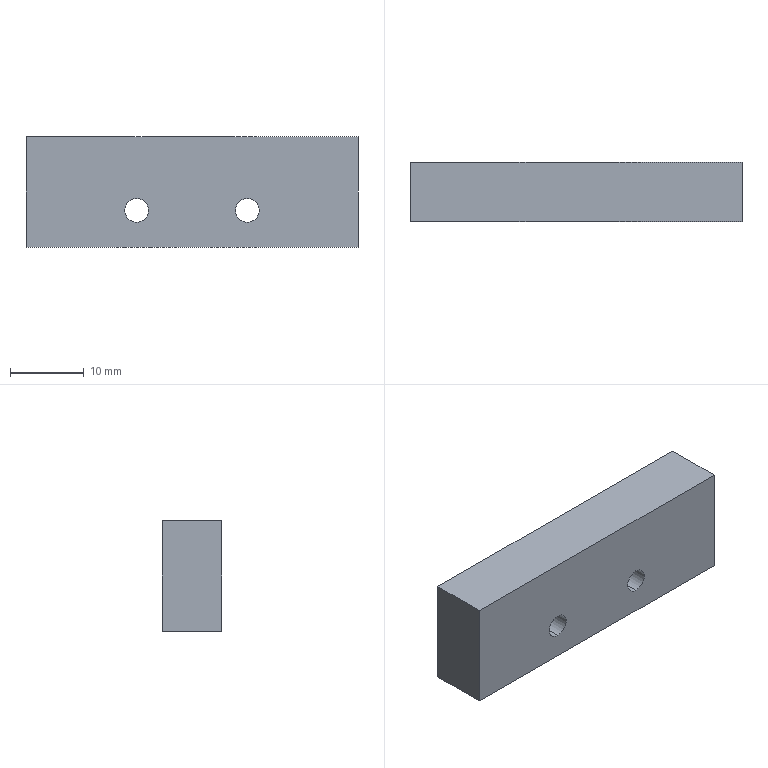Part | SolidWorks | features Extrusion 1, HoleWzd 1, ICE 1 | 1 solid | 16 faces | box 45 x 8 x 15 mm | volume 5130 mm3 | cylinder 8 | plane 8 | commonest cylinder face diameters 3.2 x4 6 x4
STEP:
#1=CARTESIAN_POINT('',(-7.5,4.5,-3.));
#2=VERTEX_POINT('',#1);
#3=CARTESIAN_POINT('',(-7.5,4.5,3.));
#4=VERTEX_POINT('',#3);
#5=CARTESIAN_POINT('',(-7.5,4.5,0.));
#6=DIRECTION('',(0.,1.,0.));
#7=DIRECTION('',(0.,0.,1.));
#8=AXIS2_PLACEMENT_3D('',#5,#6,#7);
#9=CIRCLE('',#8,3.);
#10=EDGE_CURVE('',#2,#4,#9,.T.);
#11=ORIENTED_EDGE('',*,*,#10,.F.);
#12=CARTESIAN_POINT('',(-7.5,8.,-3.));
#13=VERTEX_POINT('',#12);
#14=CARTESIAN_POINT('',(-7.5,8.,-3.));
#15=DIRECTION('',(0.,1.,0.));
#16=VECTOR('',#15,1000.);
#17=LINE('',#14,#16);
#18=EDGE_CURVE('',#2,#13,#17,.T.);
#19=ORIENTED_EDGE('',*,*,#18,.T.);
#20=CARTESIAN_POINT('',(-7.5,8.,3.));
#21=VERTEX_POINT('',#20);
#22=CARTESIAN_POINT('',(-7.5,8.,0.));
#23=DIRECTION('',(0.,1.,0.));
#24=DIRECTION('',(0.,0.,1.));
#25=AXIS2_PLACEMENT_3D('',#22,#23,#24);
#26=CIRCLE('',#25,3.);
#27=EDGE_CURVE('',#13,#21,#26,.T.);
#28=ORIENTED_EDGE('',*,*,#27,.T.);
#29=CARTESIAN_POINT('',(-7.5,8.,3.));
#30=DIRECTION('',(0.,1.,0.));
#31=VECTOR('',#30,1000.);
#32=LINE('',#29,#31);
#33=EDGE_CURVE('',#4,#21,#32,.T.);
#34=ORIENTED_EDGE('',*,*,#33,.F.);
#35=EDGE_LOOP('',(#11,#19,#28,#34));
#36=FACE_OUTER_BOUND('',#35,.T.);
#37=CARTESIAN_POINT('',(-7.5,8.,0.));
#38=DIRECTION('',(0.,1.,0.));
#39=DIRECTION('',(0.,0.,1.));
#40=AXIS2_PLACEMENT_3D('',#37,#38,#39);
#41=CYLINDRICAL_SURFACE('',#40,3.);
#42=ADVANCED_FACE('',(#36),#41,.F.);
#43=CARTESIAN_POINT('',(-7.5,0.,-1.6));
#44=VERTEX_POINT('',#43);
#45=CARTESIAN_POINT('',(-7.5,0.,1.6));
#46=VERTEX_POINT('',#45);
#47=CARTESIAN_POINT('',(-7.5,0.,0.));
#48=DIRECTION('',(0.,1.,0.));
#49=DIRECTION('',(0.,0.,1.));
#50=AXIS2_PLACEMENT_3D('',#47,#48,#49);
#51=CIRCLE('',#50,1.6);
#52=EDGE_CURVE('',#44,#46,#51,.T.);
#53=ORIENTED_EDGE('',*,*,#52,.F.);
#54=CARTESIAN_POINT('',(-7.5,4.5,-1.6));
#55=VERTEX_POINT('',#54);
#56=CARTESIAN_POINT('',(-7.5,8.,-1.6));
#57=DIRECTION('',(0.,1.,0.));
#58=VECTOR('',#57,1000.);
#59=LINE('',#56,#58);
#60=EDGE_CURVE('',#44,#55,#59,.T.);
#61=ORIENTED_EDGE('',*,*,#60,.T.);
#62=CARTESIAN_POINT('',(-7.5,4.5,1.6));
#63=VERTEX_POINT('',#62);
#64=CARTESIAN_POINT('',(-7.5,4.5,0.));
#65=DIRECTION('',(0.,1.,0.));
#66=DIRECTION('',(0.,0.,1.));
#67=AXIS2_PLACEMENT_3D('',#64,#65,#66);
#68=CIRCLE('',#67,1.6);
#69=EDGE_CURVE('',#55,#63,#68,.T.);
#70=ORIENTED_EDGE('',*,*,#69,.T.);
#71=CARTESIAN_POINT('',(-7.5,8.,1.6));
#72=DIRECTION('',(0.,1.,0.));
#73=VECTOR('',#72,1000.);
#74=LINE('',#71,#73);
#75=EDGE_CURVE('',#46,#63,#74,.T.);
#76=ORIENTED_EDGE('',*,*,#75,.F.);
#77=EDGE_LOOP('',(#53,#61,#70,#76));
#78=FACE_OUTER_BOUND('',#77,.T.);
#79=CARTESIAN_POINT('',(-7.5,8.,0.));
#80=DIRECTION('',(0.,1.,0.));
#81=DIRECTION('',(0.,0.,1.));
#82=AXIS2_PLACEMENT_3D('',#79,#80,#81);
#83=CYLINDRICAL_SURFACE('',#82,1.6);
#84=ADVANCED_FACE('',(#78),#83,.F.);
#85=CARTESIAN_POINT('',(7.5,4.5,-3.));
#86=VERTEX_POINT('',#85);
#87=CARTESIAN_POINT('',(7.5,4.5,3.));
#88=VERTEX_POINT('',#87);
#89=CARTESIAN_POINT('',(7.5,4.5,0.));
#90=DIRECTION('',(0.,1.,0.));
#91=DIRECTION('',(0.,0.,1.));
#92=AXIS2_PLACEMENT_3D('',#89,#90,#91);
#93=CIRCLE('',#92,3.);
#94=EDGE_CURVE('',#86,#88,#93,.T.);
#95=ORIENTED_EDGE('',*,*,#94,.F.);
#96=CARTESIAN_POINT('',(7.5,8.,-3.));
#97=VERTEX_POINT('',#96);
#98=CARTESIAN_POINT('',(7.5,8.,-3.));
#99=DIRECTION('',(0.,1.,0.));
#100=VECTOR('',#99,1000.);
#101=LINE('',#98,#100);
#102=EDGE_CURVE('',#86,#97,#101,.T.);
#103=ORIENTED_EDGE('',*,*,#102,.T.);
#104=CARTESIAN_POINT('',(7.5,8.,3.));
#105=VERTEX_POINT('',#104);
#106=CARTESIAN_POINT('',(7.5,8.,0.));
#107=DIRECTION('',(0.,1.,0.));
#108=DIRECTION('',(0.,0.,1.));
#109=AXIS2_PLACEMENT_3D('',#106,#107,#108);
#110=CIRCLE('',#109,3.);
#111=EDGE_CURVE('',#97,#105,#110,.T.);
#112=ORIENTED_EDGE('',*,*,#111,.T.);
#113=CARTESIAN_POINT('',(7.5,8.,3.));
#114=DIRECTION('',(0.,1.,0.));
#115=VECTOR('',#114,1000.);
#116=LINE('',#113,#115);
#117=EDGE_CURVE('',#88,#105,#116,.T.);
#118=ORIENTED_EDGE('',*,*,#117,.F.);
#119=EDGE_LOOP('',(#95,#103,#112,#118));
#120=FACE_OUTER_BOUND('',#119,.T.);
#121=CARTESIAN_POINT('',(7.5,8.,0.));
#122=DIRECTION('',(0.,1.,0.));
#123=DIRECTION('',(0.,0.,1.));
#124=AXIS2_PLACEMENT_3D('',#121,#122,#123);
#125=CYLINDRICAL_SURFACE('',#124,3.);
#126=ADVANCED_FACE('',(#120),#125,.F.);
#127=CARTESIAN_POINT('',(7.5,0.,-1.6));
#128=VERTEX_POINT('',#127);
#129=CARTESIAN_POINT('',(7.5,0.,1.6));
#130=VERTEX_POINT('',#129);
#131=CARTESIAN_POINT('',(7.5,0.,0.));
#132=DIRECTION('',(0.,1.,0.));
#133=DIRECTION('',(0.,0.,1.));
#134=AXIS2_PLACEMENT_3D('',#131,#132,#133);
#135=CIRCLE('',#134,1.6);
#136=EDGE_CURVE('',#128,#130,#135,.T.);
#137=ORIENTED_EDGE('',*,*,#136,.F.);
#138=CARTESIAN_POINT('',(7.5,4.5,-1.6));
#139=VERTEX_POINT('',#138);
#140=CARTESIAN_POINT('',(7.5,8.,-1.6));
#141=DIRECTION('',(0.,1.,0.));
#142=VECTOR('',#141,1000.);
#143=LINE('',#140,#142);
#144=EDGE_CURVE('',#128,#139,#143,.T.);
#145=ORIENTED_EDGE('',*,*,#144,.T.);
#146=CARTESIAN_POINT('',(7.5,4.5,1.6));
#147=VERTEX_POINT('',#146);
#148=CARTESIAN_POINT('',(7.5,4.5,0.));
#149=DIRECTION('',(0.,1.,0.));
#150=DIRECTION('',(0.,0.,1.));
#151=AXIS2_PLACEMENT_3D('',#148,#149,#150);
#152=CIRCLE('',#151,1.6);
#153=EDGE_CURVE('',#139,#147,#152,.T.);
#154=ORIENTED_EDGE('',*,*,#153,.T.);
#155=CARTESIAN_POINT('',(7.5,8.,1.6));
#156=DIRECTION('',(0.,1.,0.));
#157=VECTOR('',#156,1000.);
#158=LINE('',#155,#157);
#159=EDGE_CURVE('',#130,#147,#158,.T.);
#160=ORIENTED_EDGE('',*,*,#159,.F.);
#161=EDGE_LOOP('',(#137,#145,#154,#160));
#162=FACE_OUTER_BOUND('',#161,.T.);
#163=CARTESIAN_POINT('',(7.5,8.,0.));
#164=DIRECTION('',(0.,1.,0.));
#165=DIRECTION('',(0.,0.,1.));
#166=AXIS2_PLACEMENT_3D('',#163,#164,#165);
#167=CYLINDRICAL_SURFACE('',#166,1.6);
#168=ADVANCED_FACE('',(#162),#167,.F.);
#169=CARTESIAN_POINT('',(22.5,0.,10.));
#170=VERTEX_POINT('',#169);
#171=CARTESIAN_POINT('',(22.5,0.,-5.));
#172=VERTEX_POINT('',#171);
#173=CARTESIAN_POINT('',(22.5,0.,-5.));
#174=DIRECTION('',(0.,0.,-1.));
#175=VECTOR('',#174,1000.);
#176=LINE('',#173,#175);
#177=EDGE_CURVE('',#170,#172,#176,.T.);
#178=ORIENTED_EDGE('',*,*,#177,.T.);
#179=CARTESIAN_POINT('',(22.5,8.,-5.));
#180=VERTEX_POINT('',#179);
#181=CARTESIAN_POINT('',(22.5,8.,-5.));
#182=DIRECTION('',(0.,-1.,0.));
#183=VECTOR('',#182,1000.);
#184=LINE('',#181,#183);
#185=EDGE_CURVE('',#180,#172,#184,.T.);
#186=ORIENTED_EDGE('',*,*,#185,.F.);
#187=CARTESIAN_POINT('',(22.5,8.,10.));
#188=VERTEX_POINT('',#187);
#189=CARTESIAN_POINT('',(22.5,8.,-5.));
#190=DIRECTION('',(0.,0.,-1.));
#191=VECTOR('',#190,1000.);
#192=LINE('',#189,#191);
#193=EDGE_CURVE('',#188,#180,#192,.T.);
#194=ORIENTED_EDGE('',*,*,#193,.F.);
#195=CARTESIAN_POINT('',(22.5,0.,10.));
#196=DIRECTION('',(0.,1.,0.));
#197=VECTOR('',#196,1000.);
#198=LINE('',#195,#197);
#199=EDGE_CURVE('',#170,#188,#198,.T.);
#200=ORIENTED_EDGE('',*,*,#199,.F.);
#201=EDGE_LOOP('',(#178,#186,#194,#200));
#202=FACE_OUTER_BOUND('',#201,.T.);
#203=CARTESIAN_POINT('',(22.5,8.,-5.));
#204=DIRECTION('',(-1.,0.,0.));
#205=DIRECTION('',(0.,0.,1.));
#206=AXIS2_PLACEMENT_3D('',#203,#204,#205);
#207=PLANE('',#206);
#208=ADVANCED_FACE('',(#202),#207,.F.);
#209=CARTESIAN_POINT('',(-22.5,0.,-5.));
#210=VERTEX_POINT('',#209);
#211=CARTESIAN_POINT('',(-22.5,0.,-5.));
#212=DIRECTION('',(-1.,0.,0.));
#213=VECTOR('',#212,1000.);
#214=LINE('',#211,#213);
#215=EDGE_CURVE('',#172,#210,#214,.T.);
#216=ORIENTED_EDGE('',*,*,#215,.T.);
#217=CARTESIAN_POINT('',(-22.5,8.,-5.));
#218=VERTEX_POINT('',#217);
#219=CARTESIAN_POINT('',(-22.5,8.,-5.));
#220=DIRECTION('',(0.,-1.,0.));
#221=VECTOR('',#220,1000.);
#222=LINE('',#219,#221);
#223=EDGE_CURVE('',#218,#210,#222,.T.);
#224=ORIENTED_EDGE('',*,*,#223,.F.);
#225=CARTESIAN_POINT('',(-22.5,8.,-5.));
#226=DIRECTION('',(-1.,0.,0.));
#227=VECTOR('',#226,1000.);
#228=LINE('',#225,#227);
#229=EDGE_CURVE('',#180,#218,#228,.T.);
#230=ORIENTED_EDGE('',*,*,#229,.F.);
#231=ORIENTED_EDGE('',*,*,#185,.T.);
#232=EDGE_LOOP('',(#216,#224,#230,#231));
#233=FACE_OUTER_BOUND('',#232,.T.);
#234=CARTESIAN_POINT('',(-22.5,8.,-5.));
#235=DIRECTION('',(0.,0.,1.));
#236=DIRECTION('',(1.,0.,0.));
#237=AXIS2_PLACEMENT_3D('',#234,#235,#236);
#238=PLANE('',#237);
#239=ADVANCED_FACE('',(#233),#238,.F.);
#240=CARTESIAN_POINT('',(-22.5,0.,10.));
#241=VERTEX_POINT('',#240);
#242=CARTESIAN_POINT('',(-22.5,0.,-5.));
#243=DIRECTION('',(0.,0.,1.));
#244=VECTOR('',#243,1000.);
#245=LINE('',#242,#244);
#246=EDGE_CURVE('',#210,#241,#245,.T.);
#247=ORIENTED_EDGE('',*,*,#246,.T.);
#248=CARTESIAN_POINT('',(-22.5,8.,10.));
#249=VERTEX_POINT('',#248);
#250=CARTESIAN_POINT('',(-22.5,8.,10.));
#251=DIRECTION('',(0.,-1.,0.));
#252=VECTOR('',#251,1000.);
#253=LINE('',#250,#252);
#254=EDGE_CURVE('',#249,#241,#253,.T.);
#255=ORIENTED_EDGE('',*,*,#254,.F.);
#256=CARTESIAN_POINT('',(-22.5,8.,-5.));
#257=DIRECTION('',(0.,0.,1.));
#258=VECTOR('',#257,1000.);
#259=LINE('',#256,#258);
#260=EDGE_CURVE('',#218,#249,#259,.T.);
#261=ORIENTED_EDGE('',*,*,#260,.F.);
#262=ORIENTED_EDGE('',*,*,#223,.T.);
#263=EDGE_LOOP('',(#247,#255,#261,#262));
#264=FACE_OUTER_BOUND('',#263,.T.);
#265=CARTESIAN_POINT('',(-22.5,8.,-5.));
#266=DIRECTION('',(1.,0.,0.));
#267=DIRECTION('',(0.,0.,-1.));
#268=AXIS2_PLACEMENT_3D('',#265,#266,#267);
#269=PLANE('',#268);
#270=ADVANCED_FACE('',(#264),#269,.F.);
#271=CARTESIAN_POINT('',(-7.5,8.,0.));
#272=DIRECTION('',(0.,1.,0.));
#273=DIRECTION('',(0.,0.,1.));
#274=AXIS2_PLACEMENT_3D('',#271,#272,#273);
#275=CIRCLE('',#274,3.);
#276=EDGE_CURVE('',#21,#13,#275,.T.);
#277=ORIENTED_EDGE('',*,*,#276,.F.);
#278=ORIENTED_EDGE('',*,*,#27,.F.);
#279=EDGE_LOOP('',(#277,#278));
#280=FACE_BOUND('',#279,.T.);
#281=CARTESIAN_POINT('',(7.5,8.,0.));
#282=DIRECTION('',(0.,1.,0.));
#283=DIRECTION('',(0.,0.,1.));
#284=AXIS2_PLACEMENT_3D('',#281,#282,#283);
#285=CIRCLE('',#284,3.);
#286=EDGE_CURVE('',#105,#97,#285,.T.);
#287=ORIENTED_EDGE('',*,*,#286,.F.);
#288=ORIENTED_EDGE('',*,*,#111,.F.);
#289=EDGE_LOOP('',(#287,#288));
#290=FACE_BOUND('',#289,.T.);
#291=ORIENTED_EDGE('',*,*,#193,.T.);
#292=ORIENTED_EDGE('',*,*,#229,.T.);
#293=ORIENTED_EDGE('',*,*,#260,.T.);
#294=CARTESIAN_POINT('',(22.5,8.,10.));
#295=DIRECTION('',(-1.,0.,0.));
#296=VECTOR('',#295,1000.);
#297=LINE('',#294,#296);
#298=EDGE_CURVE('',#188,#249,#297,.T.);
#299=ORIENTED_EDGE('',*,*,#298,.F.);
#300=EDGE_LOOP('',(#291,#292,#293,#299));
#301=FACE_OUTER_BOUND('',#300,.T.);
#302=CARTESIAN_POINT('',(0.,8.,0.));
#303=DIRECTION('',(0.,1.,0.));
#304=DIRECTION('',(0.,0.,1.));
#305=AXIS2_PLACEMENT_3D('',#302,#303,#304);
#306=PLANE('',#305);
#307=ADVANCED_FACE('',(#280,#290,#301),#306,.T.);
#308=CARTESIAN_POINT('',(-7.5,0.,0.));
#309=DIRECTION('',(0.,1.,0.));
#310=DIRECTION('',(0.,0.,1.));
#311=AXIS2_PLACEMENT_3D('',#308,#309,#310);
#312=CIRCLE('',#311,1.6);
#313=EDGE_CURVE('',#46,#44,#312,.T.);
#314=ORIENTED_EDGE('',*,*,#313,.T.);
#315=ORIENTED_EDGE('',*,*,#52,.T.);
#316=EDGE_LOOP('',(#314,#315));
#317=FACE_BOUND('',#316,.T.);
#318=CARTESIAN_POINT('',(7.5,0.,0.));
#319=DIRECTION('',(0.,1.,0.));
#320=DIRECTION('',(0.,0.,1.));
#321=AXIS2_PLACEMENT_3D('',#318,#319,#320);
#322=CIRCLE('',#321,1.6);
#323=EDGE_CURVE('',#130,#128,#322,.T.);
#324=ORIENTED_EDGE('',*,*,#323,.T.);
#325=ORIENTED_EDGE('',*,*,#136,.T.);
#326=EDGE_LOOP('',(#324,#325));
#327=FACE_BOUND('',#326,.T.);
#328=ORIENTED_EDGE('',*,*,#177,.F.);
#329=CARTESIAN_POINT('',(-22.5,0.,10.));
#330=DIRECTION('',(1.,0.,0.));
#331=VECTOR('',#330,1000.);
#332=LINE('',#329,#331);
#333=EDGE_CURVE('',#241,#170,#332,.T.);
#334=ORIENTED_EDGE('',*,*,#333,.F.);
#335=ORIENTED_EDGE('',*,*,#246,.F.);
#336=ORIENTED_EDGE('',*,*,#215,.F.);
#337=EDGE_LOOP('',(#328,#334,#335,#336));
#338=FACE_OUTER_BOUND('',#337,.T.);
#339=CARTESIAN_POINT('',(0.,0.,0.));
#340=DIRECTION('',(0.,1.,0.));
#341=DIRECTION('',(0.,0.,1.));
#342=AXIS2_PLACEMENT_3D('',#339,#340,#341);
#343=PLANE('',#342);
#344=ADVANCED_FACE('',(#317,#327,#338),#343,.F.);
#345=ORIENTED_EDGE('',*,*,#144,.F.);
#346=ORIENTED_EDGE('',*,*,#323,.F.);
#347=ORIENTED_EDGE('',*,*,#159,.T.);
#348=CARTESIAN_POINT('',(7.5,4.5,0.));
#349=DIRECTION('',(0.,1.,0.));
#350=DIRECTION('',(0.,0.,1.));
#351=AXIS2_PLACEMENT_3D('',#348,#349,#350);
#352=CIRCLE('',#351,1.6);
#353=EDGE_CURVE('',#147,#139,#352,.T.);
#354=ORIENTED_EDGE('',*,*,#353,.T.);
#355=EDGE_LOOP('',(#345,#346,#347,#354));
#356=FACE_OUTER_BOUND('',#355,.T.);
#357=CARTESIAN_POINT('',(7.5,8.,0.));
#358=DIRECTION('',(0.,1.,0.));
#359=DIRECTION('',(0.,0.,1.));
#360=AXIS2_PLACEMENT_3D('',#357,#358,#359);
#361=CYLINDRICAL_SURFACE('',#360,1.6);
#362=ADVANCED_FACE('',(#356),#361,.F.);
#363=ORIENTED_EDGE('',*,*,#353,.F.);
#364=ORIENTED_EDGE('',*,*,#153,.F.);
#365=EDGE_LOOP('',(#363,#364));
#366=FACE_BOUND('',#365,.T.);
#367=CARTESIAN_POINT('',(7.5,4.5,0.));
#368=DIRECTION('',(0.,1.,0.));
#369=DIRECTION('',(0.,0.,1.));
#370=AXIS2_PLACEMENT_3D('',#367,#368,#369);
#371=CIRCLE('',#370,3.);
#372=EDGE_CURVE('',#88,#86,#371,.T.);
#373=ORIENTED_EDGE('',*,*,#372,.T.);
#374=ORIENTED_EDGE('',*,*,#94,.T.);
#375=EDGE_LOOP('',(#373,#374));
#376=FACE_OUTER_BOUND('',#375,.T.);
#377=CARTESIAN_POINT('',(9.1,4.5,0.));
#378=DIRECTION('',(0.,-1.,0.));
#379=DIRECTION('',(0.,0.,-1.));
#380=AXIS2_PLACEMENT_3D('',#377,#378,#379);
#381=PLANE('',#380);
#382=ADVANCED_FACE('',(#366,#376),#381,.F.);
#383=ORIENTED_EDGE('',*,*,#102,.F.);
#384=ORIENTED_EDGE('',*,*,#372,.F.);
#385=ORIENTED_EDGE('',*,*,#117,.T.);
#386=ORIENTED_EDGE('',*,*,#286,.T.);
#387=EDGE_LOOP('',(#383,#384,#385,#386));
#388=FACE_OUTER_BOUND('',#387,.T.);
#389=CARTESIAN_POINT('',(7.5,8.,0.));
#390=DIRECTION('',(0.,1.,0.));
#391=DIRECTION('',(0.,0.,1.));
#392=AXIS2_PLACEMENT_3D('',#389,#390,#391);
#393=CYLINDRICAL_SURFACE('',#392,3.);
#394=ADVANCED_FACE('',(#388),#393,.F.);
#395=ORIENTED_EDGE('',*,*,#60,.F.);
#396=ORIENTED_EDGE('',*,*,#313,.F.);
#397=ORIENTED_EDGE('',*,*,#75,.T.);
#398=CARTESIAN_POINT('',(-7.5,4.5,0.));
#399=DIRECTION('',(0.,1.,0.));
#400=DIRECTION('',(0.,0.,1.));
#401=AXIS2_PLACEMENT_3D('',#398,#399,#400);
#402=CIRCLE('',#401,1.6);
#403=EDGE_CURVE('',#63,#55,#402,.T.);
#404=ORIENTED_EDGE('',*,*,#403,.T.);
#405=EDGE_LOOP('',(#395,#396,#397,#404));
#406=FACE_OUTER_BOUND('',#405,.T.);
#407=CARTESIAN_POINT('',(-7.5,8.,0.));
#408=DIRECTION('',(0.,1.,0.));
#409=DIRECTION('',(0.,0.,1.));
#410=AXIS2_PLACEMENT_3D('',#407,#408,#409);
#411=CYLINDRICAL_SURFACE('',#410,1.6);
#412=ADVANCED_FACE('',(#406),#411,.F.);
#413=ORIENTED_EDGE('',*,*,#403,.F.);
#414=ORIENTED_EDGE('',*,*,#69,.F.);
#415=EDGE_LOOP('',(#413,#414));
#416=FACE_BOUND('',#415,.T.);
#417=CARTESIAN_POINT('',(-7.5,4.5,0.));
#418=DIRECTION('',(0.,1.,0.));
#419=DIRECTION('',(0.,0.,1.));
#420=AXIS2_PLACEMENT_3D('',#417,#418,#419);
#421=CIRCLE('',#420,3.);
#422=EDGE_CURVE('',#4,#2,#421,.T.);
#423=ORIENTED_EDGE('',*,*,#422,.T.);
#424=ORIENTED_EDGE('',*,*,#10,.T.);
#425=EDGE_LOOP('',(#423,#424));
#426=FACE_OUTER_BOUND('',#425,.T.);
#427=CARTESIAN_POINT('',(-5.9,4.5,0.));
#428=DIRECTION('',(0.,-1.,0.));
#429=DIRECTION('',(0.,0.,-1.));
#430=AXIS2_PLACEMENT_3D('',#427,#428,#429);
#431=PLANE('',#430);
#432=ADVANCED_FACE('',(#416,#426),#431,.F.);
#433=ORIENTED_EDGE('',*,*,#18,.F.);
#434=ORIENTED_EDGE('',*,*,#422,.F.);
#435=ORIENTED_EDGE('',*,*,#33,.T.);
#436=ORIENTED_EDGE('',*,*,#276,.T.);
#437=EDGE_LOOP('',(#433,#434,#435,#436));
#438=FACE_OUTER_BOUND('',#437,.T.);
#439=CARTESIAN_POINT('',(-7.5,8.,0.));
#440=DIRECTION('',(0.,1.,0.));
#441=DIRECTION('',(0.,0.,1.));
#442=AXIS2_PLACEMENT_3D('',#439,#440,#441);
#443=CYLINDRICAL_SURFACE('',#442,3.);
#444=ADVANCED_FACE('',(#438),#443,.F.);
#445=ORIENTED_EDGE('',*,*,#254,.T.);
#446=ORIENTED_EDGE('',*,*,#333,.T.);
#447=ORIENTED_EDGE('',*,*,#199,.T.);
#448=ORIENTED_EDGE('',*,*,#298,.T.);
#449=EDGE_LOOP('',(#445,#446,#447,#448));
#450=FACE_OUTER_BOUND('',#449,.T.);
#451=CARTESIAN_POINT('',(0.,0.,10.));
#452=DIRECTION('',(0.,0.,1.));
#453=DIRECTION('',(1.,0.,0.));
#454=AXIS2_PLACEMENT_3D('',#451,#452,#453);
#455=PLANE('',#454);
#456=ADVANCED_FACE('',(#450),#455,.T.);
#457=CLOSED_SHELL('',(#42,#84,#126,#168,#208,#239,#270,#307,#344,#362,#382,#394,#412,#432,#444,#456));
#458=MANIFOLD_SOLID_BREP('',#457);
#459=CARTESIAN_POINT('',(0.,0.,0.));
#460=DIRECTION('',(0.,0.,1.));
#461=DIRECTION('',(1.,0.,0.));
#462=AXIS2_PLACEMENT_3D('',#459,#460,#461);
#463=(LENGTH_UNIT()NAMED_UNIT(*)SI_UNIT(.MILLI.,.METRE.));
#464=UNCERTAINTY_MEASURE_WITH_UNIT(LENGTH_MEASURE(0.00001),#463,'','');
#465=(NAMED_UNIT(*)PLANE_ANGLE_UNIT()SI_UNIT($,.RADIAN.));
#466=(NAMED_UNIT(*)SI_UNIT($,.STERADIAN.)SOLID_ANGLE_UNIT());
#467=(GEOMETRIC_REPRESENTATION_CONTEXT(3)GLOBAL_UNCERTAINTY_ASSIGNED_CONTEXT((#464))GLOBAL_UNIT_ASSIGNED_CONTEXT((#463,#465,#466))REPRESENTATION_CONTEXT('',''));
#468=ADVANCED_BREP_SHAPE_REPRESENTATION('',(#458,#462),#467);